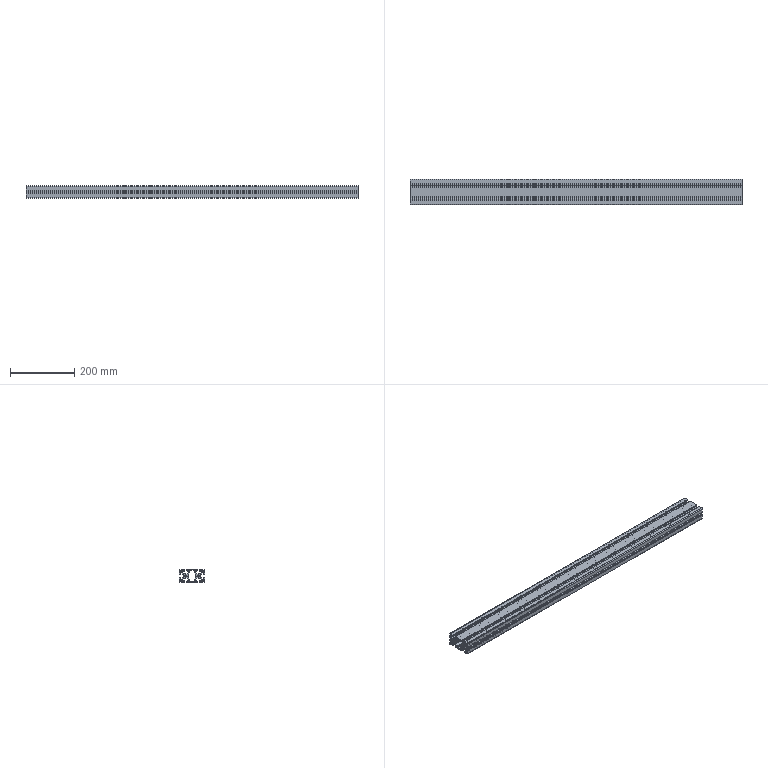Part | NX | features BREP 1 | 1 solid | 286 faces | box 1036 x 80 x 40 mm | volume 1292195 mm3 | plane 150 | cylinder 136 | commonest cylinder face diameters 1 x60 0.4 x36 4 x16 5 x8 6 x8 0.6 x4